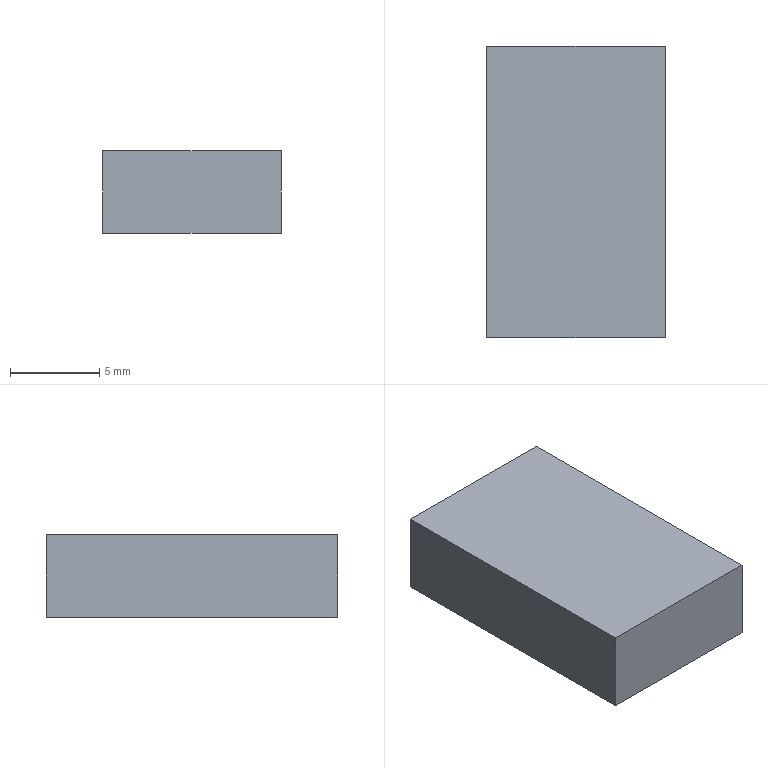Part | NX | features solid 2 | 1 solid | 6 faces | box 10 x 16.321 x 4.65 mm | volume 758.953 mm3 | plane 6
STEP:
#1=CARTESIAN_POINT('',(2250.,-341.279,-577.962));
#2=VERTEX_POINT('',#1);
#3=CARTESIAN_POINT('',(2250.,-357.6,-577.962));
#4=VERTEX_POINT('',#3);
#5=CARTESIAN_POINT('',(2250.,-341.279,-577.962));
#6=CARTESIAN_POINT('',(2250.,-346.719,-577.962));
#7=CARTESIAN_POINT('',(2250.,-352.16,-577.962));
#8=CARTESIAN_POINT('',(2250.,-357.6,-577.962));
#9=B_SPLINE_CURVE_WITH_KNOTS('',3,(#5,#6,#7,#8),.UNSPECIFIED.,.F.,.F.,(4,4),(0.,0.3891),.PIECEWISE_BEZIER_KNOTS.);
#10=EDGE_CURVE('',#2,#4,#9,.T.);
#11=ORIENTED_EDGE('',*,*,#10,.F.);
#12=CARTESIAN_POINT('',(2260.,-341.279,-577.962));
#13=VERTEX_POINT('',#12);
#14=CARTESIAN_POINT('',(2260.,-341.279,-577.962));
#15=DIRECTION('',(-1.,0.,0.));
#16=VECTOR('',#15,1000.);
#17=LINE('',#14,#16);
#18=EDGE_CURVE('',#13,#2,#17,.T.);
#19=ORIENTED_EDGE('',*,*,#18,.F.);
#20=CARTESIAN_POINT('',(2260.,-357.6,-577.962));
#21=VERTEX_POINT('',#20);
#22=CARTESIAN_POINT('',(2260.,-341.279,-577.962));
#23=CARTESIAN_POINT('',(2260.,-346.719,-577.962));
#24=CARTESIAN_POINT('',(2260.,-352.16,-577.962));
#25=CARTESIAN_POINT('',(2260.,-357.6,-577.962));
#26=B_SPLINE_CURVE_WITH_KNOTS('',3,(#22,#23,#24,#25),.UNSPECIFIED.,.F.,.F.,(4,4),(0.,0.3891),.PIECEWISE_BEZIER_KNOTS.);
#27=EDGE_CURVE('',#13,#21,#26,.T.);
#28=ORIENTED_EDGE('',*,*,#27,.T.);
#29=CARTESIAN_POINT('',(2260.,-357.6,-577.962));
#30=DIRECTION('',(-1.,0.,0.));
#31=VECTOR('',#30,1000.);
#32=LINE('',#29,#31);
#33=EDGE_CURVE('',#21,#4,#32,.T.);
#34=ORIENTED_EDGE('',*,*,#33,.T.);
#35=EDGE_LOOP('',(#11,#19,#28,#34));
#36=FACE_BOUND('',#35,.T.);
#37=CARTESIAN_POINT('',(2260.,-341.279,-577.962));
#38=DIRECTION('',(0.,0.,-1.));
#39=DIRECTION('',(-1.,0.,0.));
#40=AXIS2_PLACEMENT_3D('',#37,#38,#39);
#41=PLANE('',#40);
#42=ADVANCED_FACE('',(#36),#41,.T.);
#43=CARTESIAN_POINT('',(2250.,-357.6,-573.312));
#44=VERTEX_POINT('',#43);
#45=CARTESIAN_POINT('',(2250.,-357.6,-577.962));
#46=CARTESIAN_POINT('',(2250.,-357.6,-576.412));
#47=CARTESIAN_POINT('',(2250.,-357.6,-574.862));
#48=CARTESIAN_POINT('',(2250.,-357.6,-573.312));
#49=B_SPLINE_CURVE_WITH_KNOTS('',3,(#45,#46,#47,#48),.UNSPECIFIED.,.F.,.F.,(4,4),(0.3891,0.5),.PIECEWISE_BEZIER_KNOTS.);
#50=EDGE_CURVE('',#4,#44,#49,.T.);
#51=ORIENTED_EDGE('',*,*,#50,.F.);
#52=ORIENTED_EDGE('',*,*,#33,.F.);
#53=CARTESIAN_POINT('',(2260.,-357.6,-573.312));
#54=VERTEX_POINT('',#53);
#55=CARTESIAN_POINT('',(2260.,-357.6,-577.962));
#56=CARTESIAN_POINT('',(2260.,-357.6,-576.412));
#57=CARTESIAN_POINT('',(2260.,-357.6,-574.862));
#58=CARTESIAN_POINT('',(2260.,-357.6,-573.312));
#59=B_SPLINE_CURVE_WITH_KNOTS('',3,(#55,#56,#57,#58),.UNSPECIFIED.,.F.,.F.,(4,4),(0.3891,0.5),.PIECEWISE_BEZIER_KNOTS.);
#60=EDGE_CURVE('',#21,#54,#59,.T.);
#61=ORIENTED_EDGE('',*,*,#60,.T.);
#62=CARTESIAN_POINT('',(2260.,-357.6,-573.312));
#63=DIRECTION('',(-1.,0.,0.));
#64=VECTOR('',#63,1000.);
#65=LINE('',#62,#64);
#66=EDGE_CURVE('',#54,#44,#65,.T.);
#67=ORIENTED_EDGE('',*,*,#66,.T.);
#68=EDGE_LOOP('',(#51,#52,#61,#67));
#69=FACE_BOUND('',#68,.T.);
#70=CARTESIAN_POINT('',(2260.,-357.6,-577.962));
#71=DIRECTION('',(0.,-1.,0.));
#72=DIRECTION('',(1.,0.,0.));
#73=AXIS2_PLACEMENT_3D('',#70,#71,#72);
#74=PLANE('',#73);
#75=ADVANCED_FACE('',(#69),#74,.T.);
#76=CARTESIAN_POINT('',(2250.,-341.279,-573.312));
#77=VERTEX_POINT('',#76);
#78=CARTESIAN_POINT('',(2250.,-357.6,-573.312));
#79=CARTESIAN_POINT('',(2250.,-352.16,-573.312));
#80=CARTESIAN_POINT('',(2250.,-346.719,-573.312));
#81=CARTESIAN_POINT('',(2250.,-341.279,-573.312));
#82=B_SPLINE_CURVE_WITH_KNOTS('',3,(#78,#79,#80,#81),.UNSPECIFIED.,.F.,.F.,(4,4),(0.5,0.8891),.PIECEWISE_BEZIER_KNOTS.);
#83=EDGE_CURVE('',#44,#77,#82,.T.);
#84=ORIENTED_EDGE('',*,*,#83,.F.);
#85=ORIENTED_EDGE('',*,*,#66,.F.);
#86=CARTESIAN_POINT('',(2260.,-341.279,-573.312));
#87=VERTEX_POINT('',#86);
#88=CARTESIAN_POINT('',(2260.,-357.6,-573.312));
#89=CARTESIAN_POINT('',(2260.,-352.16,-573.312));
#90=CARTESIAN_POINT('',(2260.,-346.719,-573.312));
#91=CARTESIAN_POINT('',(2260.,-341.279,-573.312));
#92=B_SPLINE_CURVE_WITH_KNOTS('',3,(#88,#89,#90,#91),.UNSPECIFIED.,.F.,.F.,(4,4),(0.5,0.8891),.PIECEWISE_BEZIER_KNOTS.);
#93=EDGE_CURVE('',#54,#87,#92,.T.);
#94=ORIENTED_EDGE('',*,*,#93,.T.);
#95=CARTESIAN_POINT('',(2260.,-341.279,-573.312));
#96=DIRECTION('',(-1.,0.,0.));
#97=VECTOR('',#96,1000.);
#98=LINE('',#95,#97);
#99=EDGE_CURVE('',#87,#77,#98,.T.);
#100=ORIENTED_EDGE('',*,*,#99,.T.);
#101=EDGE_LOOP('',(#84,#85,#94,#100));
#102=FACE_BOUND('',#101,.T.);
#103=CARTESIAN_POINT('',(2260.,-357.6,-573.312));
#104=DIRECTION('',(0.,0.,1.));
#105=DIRECTION('',(1.,0.,0.));
#106=AXIS2_PLACEMENT_3D('',#103,#104,#105);
#107=PLANE('',#106);
#108=ADVANCED_FACE('',(#102),#107,.T.);
#109=CARTESIAN_POINT('',(2250.,-341.279,-573.312));
#110=CARTESIAN_POINT('',(2250.,-341.279,-574.862));
#111=CARTESIAN_POINT('',(2250.,-341.279,-576.412));
#112=CARTESIAN_POINT('',(2250.,-341.279,-577.962));
#113=B_SPLINE_CURVE_WITH_KNOTS('',3,(#109,#110,#111,#112),.UNSPECIFIED.,.F.,.F.,(4,4),(0.8891,1.),.PIECEWISE_BEZIER_KNOTS.);
#114=EDGE_CURVE('',#77,#2,#113,.T.);
#115=ORIENTED_EDGE('',*,*,#114,.F.);
#116=ORIENTED_EDGE('',*,*,#99,.F.);
#117=CARTESIAN_POINT('',(2260.,-341.279,-573.312));
#118=CARTESIAN_POINT('',(2260.,-341.279,-574.862));
#119=CARTESIAN_POINT('',(2260.,-341.279,-576.412));
#120=CARTESIAN_POINT('',(2260.,-341.279,-577.962));
#121=B_SPLINE_CURVE_WITH_KNOTS('',3,(#117,#118,#119,#120),.UNSPECIFIED.,.F.,.F.,(4,4),(0.8891,1.),.PIECEWISE_BEZIER_KNOTS.);
#122=EDGE_CURVE('',#87,#13,#121,.T.);
#123=ORIENTED_EDGE('',*,*,#122,.T.);
#124=ORIENTED_EDGE('',*,*,#18,.T.);
#125=EDGE_LOOP('',(#115,#116,#123,#124));
#126=FACE_BOUND('',#125,.T.);
#127=CARTESIAN_POINT('',(2260.,-341.279,-573.312));
#128=DIRECTION('',(0.,1.,0.));
#129=DIRECTION('',(-1.,0.,0.));
#130=AXIS2_PLACEMENT_3D('',#127,#128,#129);
#131=PLANE('',#130);
#132=ADVANCED_FACE('',(#126),#131,.T.);
#133=ORIENTED_EDGE('',*,*,#27,.F.);
#134=ORIENTED_EDGE('',*,*,#122,.F.);
#135=ORIENTED_EDGE('',*,*,#93,.F.);
#136=ORIENTED_EDGE('',*,*,#60,.F.);
#137=EDGE_LOOP('',(#133,#134,#135,#136));
#138=FACE_BOUND('',#137,.T.);
#139=CARTESIAN_POINT('',(2260.,-349.439,-577.962));
#140=DIRECTION('',(1.,0.,0.));
#141=DIRECTION('',(0.,1.,0.));
#142=AXIS2_PLACEMENT_3D('',#139,#140,#141);
#143=PLANE('',#142);
#144=ADVANCED_FACE('',(#138),#143,.T.);
#145=ORIENTED_EDGE('',*,*,#10,.T.);
#146=ORIENTED_EDGE('',*,*,#50,.T.);
#147=ORIENTED_EDGE('',*,*,#83,.T.);
#148=ORIENTED_EDGE('',*,*,#114,.T.);
#149=EDGE_LOOP('',(#145,#146,#147,#148));
#150=FACE_BOUND('',#149,.T.);
#151=CARTESIAN_POINT('',(2250.,-349.439,-577.962));
#152=DIRECTION('',(1.,0.,0.));
#153=DIRECTION('',(0.,1.,0.));
#154=AXIS2_PLACEMENT_3D('',#151,#152,#153);
#155=PLANE('',#154);
#156=ADVANCED_FACE('',(#150),#155,.F.);
#157=CLOSED_SHELL('',(#42,#75,#108,#132,#144,#156));
#158=MANIFOLD_SOLID_BREP('',#157);
#159=(LENGTH_UNIT()NAMED_UNIT(*)SI_UNIT(.MILLI.,.METRE.));
#160=UNCERTAINTY_MEASURE_WITH_UNIT(LENGTH_MEASURE(0.00001),#159,'','');
#161=(NAMED_UNIT(*)PLANE_ANGLE_UNIT()SI_UNIT($,.RADIAN.));
#162=(NAMED_UNIT(*)SI_UNIT($,.STERADIAN.)SOLID_ANGLE_UNIT());
#163=(GEOMETRIC_REPRESENTATION_CONTEXT(3)GLOBAL_UNCERTAINTY_ASSIGNED_CONTEXT((#160))GLOBAL_UNIT_ASSIGNED_CONTEXT((#159,#161,#162))REPRESENTATION_CONTEXT('',''));
#164=ADVANCED_BREP_SHAPE_REPRESENTATION('',(#158),#163);